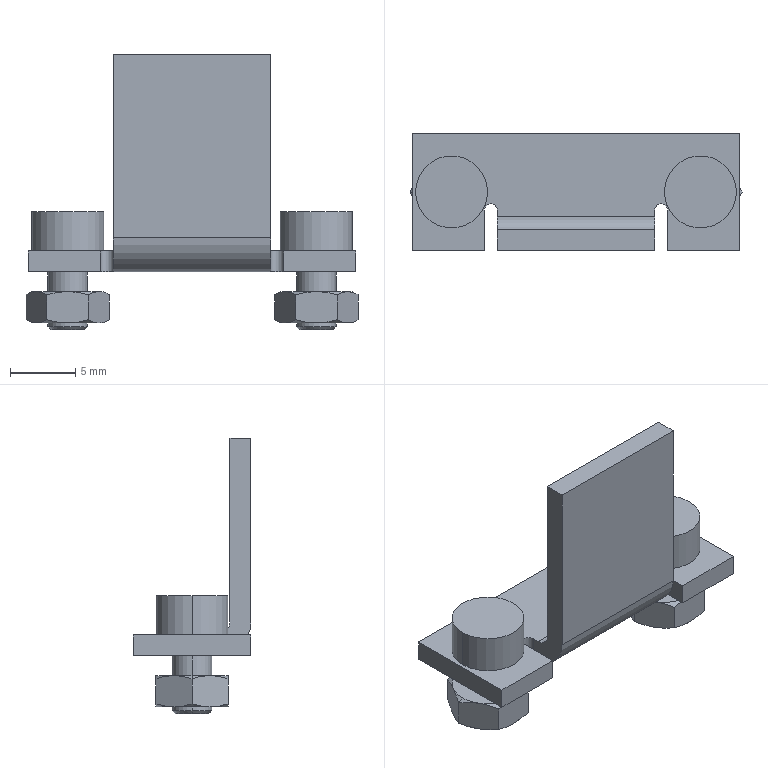Part | STEP file | QA-PHOTO_SENSOR_br | 1 solid | 82 faces | box 25.351 x 9 x 21 mm | volume 917.475 mm3 | plane 34 | cone 32 | cylinder 16 | commonest cylinder face diameters 3 x8 5.5 x4 1 x2 2 x1 5.2 x1